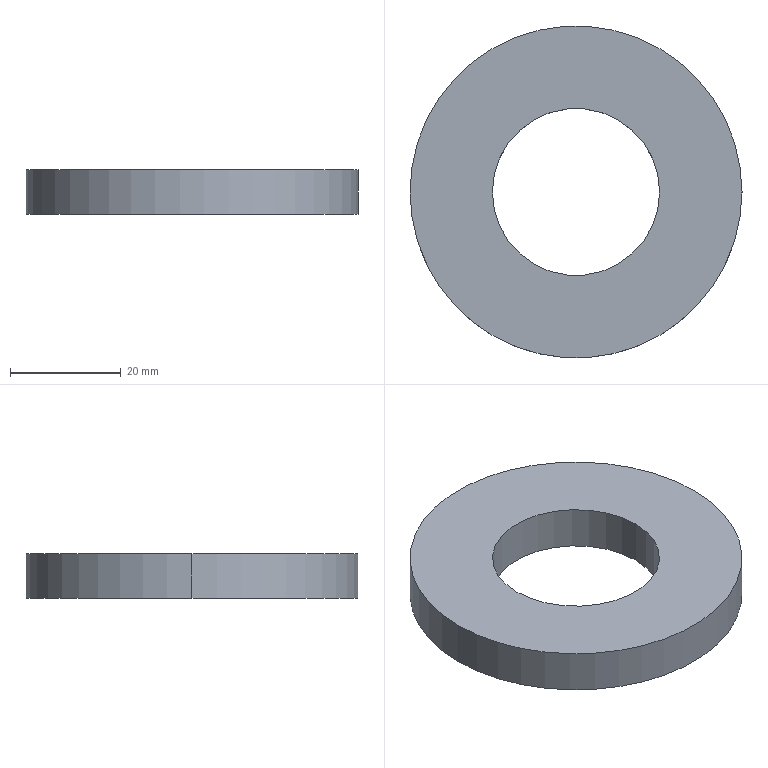Part | STEP file | LM-05-1237_default | 1 solid | 6 faces | box 60 x 60 x 8 mm | volume 16889 mm3 | cylinder 4 | plane 2 | commonest cylinder face diameters 30.2 x2 60 x2
STEP:
#1=CARTESIAN_POINT('',(0.,0.,0.));
#2=DIRECTION('',(0.,0.,1.));
#3=DIRECTION('',(1.,0.,0.));
#4=AXIS2_PLACEMENT_3D('',#1,#2,#3);
#5=CARTESIAN_POINT('',(-15.1,0.,4.));
#6=VERTEX_POINT('',#5);
#7=CARTESIAN_POINT('',(-15.1,0.,-4.));
#8=VERTEX_POINT('',#7);
#9=CARTESIAN_POINT('',(-15.1,0.,4.));
#10=DIRECTION('',(0.,0.,-1.));
#11=VECTOR('',#10,1.);
#12=LINE('',#9,#11);
#13=CARTESIAN_POINT('',(0.,0.,4.));
#14=DIRECTION('',(0.,0.,-1.));
#15=DIRECTION('',(-1.,0.,0.));
#16=AXIS2_PLACEMENT_3D('',#13,#14,#15);
#17=CYLINDRICAL_SURFACE('',#16,15.1);
#18=CARTESIAN_POINT('',(6.283,0.));
#19=DIRECTION('',(0.,1.));
#20=VECTOR('',#19,1.);
#21=LINE('',#18,#20);
#22=(GEOMETRIC_REPRESENTATION_CONTEXT(2)PARAMETRIC_REPRESENTATION_CONTEXT()REPRESENTATION_CONTEXT('',''));
#23=DEFINITIONAL_REPRESENTATION('',(#21),#22);
#24=PCURVE('',#17,#23);
#25=CARTESIAN_POINT('',(0.,0.,4.));
#26=DIRECTION('',(0.,0.,-1.));
#27=DIRECTION('',(-1.,0.,0.));
#28=AXIS2_PLACEMENT_3D('',#25,#26,#27);
#29=CYLINDRICAL_SURFACE('',#28,15.1);
#30=CARTESIAN_POINT('',(0.,0.));
#31=DIRECTION('',(0.,1.));
#32=VECTOR('',#31,1.);
#33=LINE('',#30,#32);
#34=(GEOMETRIC_REPRESENTATION_CONTEXT(2)PARAMETRIC_REPRESENTATION_CONTEXT()REPRESENTATION_CONTEXT('',''));
#35=DEFINITIONAL_REPRESENTATION('',(#33),#34);
#36=PCURVE('',#29,#35);
#37=SURFACE_CURVE('',#12,(#24,#36),.PCURVE_S1.);
#38=EDGE_CURVE('',#6,#8,#37,.T.);
#39=ORIENTED_EDGE('',*,*,#38,.T.);
#40=CARTESIAN_POINT('',(15.1,0.,-4.));
#41=VERTEX_POINT('',#40);
#42=CARTESIAN_POINT('',(0.,0.,-4.));
#43=DIRECTION('',(0.,0.,1.));
#44=DIRECTION('',(1.,0.,0.));
#45=AXIS2_PLACEMENT_3D('',#42,#43,#44);
#46=CIRCLE('',#45,15.1);
#47=CARTESIAN_POINT('',(9.425,8.));
#48=DIRECTION('',(-1.,0.));
#49=VECTOR('',#48,1.);
#50=LINE('',#47,#49);
#51=(GEOMETRIC_REPRESENTATION_CONTEXT(2)PARAMETRIC_REPRESENTATION_CONTEXT()REPRESENTATION_CONTEXT('',''));
#52=DEFINITIONAL_REPRESENTATION('',(#50),#51);
#53=PCURVE('',#17,#52);
#54=CARTESIAN_POINT('',(0.,0.,-4.));
#55=DIRECTION('',(0.,0.,1.));
#56=DIRECTION('',(1.,0.,0.));
#57=AXIS2_PLACEMENT_3D('',#54,#55,#56);
#58=PLANE('',#57);
#59=CARTESIAN_POINT('',(0.,0.));
#60=DIRECTION('',(1.,0.));
#61=AXIS2_PLACEMENT_2D('',#59,#60);
#62=CIRCLE('',#61,15.1);
#63=(GEOMETRIC_REPRESENTATION_CONTEXT(2)PARAMETRIC_REPRESENTATION_CONTEXT()REPRESENTATION_CONTEXT('',''));
#64=DEFINITIONAL_REPRESENTATION('',(#62),#63);
#65=PCURVE('',#58,#64);
#66=SURFACE_CURVE('',#46,(#53,#65),.PCURVE_S1.);
#67=EDGE_CURVE('',#8,#41,#66,.T.);
#68=ORIENTED_EDGE('',*,*,#67,.T.);
#69=CARTESIAN_POINT('',(15.1,0.,4.));
#70=VERTEX_POINT('',#69);
#71=CARTESIAN_POINT('',(15.1,0.,4.));
#72=DIRECTION('',(0.,0.,-1.));
#73=VECTOR('',#72,1.);
#74=LINE('',#71,#73);
#75=CARTESIAN_POINT('',(3.142,0.));
#76=DIRECTION('',(0.,1.));
#77=VECTOR('',#76,1.);
#78=LINE('',#75,#77);
#79=(GEOMETRIC_REPRESENTATION_CONTEXT(2)PARAMETRIC_REPRESENTATION_CONTEXT()REPRESENTATION_CONTEXT('',''));
#80=DEFINITIONAL_REPRESENTATION('',(#78),#79);
#81=PCURVE('',#17,#80);
#82=CARTESIAN_POINT('',(3.142,0.));
#83=DIRECTION('',(0.,1.));
#84=VECTOR('',#83,1.);
#85=LINE('',#82,#84);
#86=(GEOMETRIC_REPRESENTATION_CONTEXT(2)PARAMETRIC_REPRESENTATION_CONTEXT()REPRESENTATION_CONTEXT('',''));
#87=DEFINITIONAL_REPRESENTATION('',(#85),#86);
#88=PCURVE('',#29,#87);
#89=SURFACE_CURVE('',#74,(#81,#88),.PCURVE_S1.);
#90=EDGE_CURVE('',#70,#41,#89,.T.);
#91=ORIENTED_EDGE('',*,*,#90,.F.);
#92=CARTESIAN_POINT('',(0.,0.,4.));
#93=DIRECTION('',(0.,0.,1.));
#94=DIRECTION('',(1.,0.,0.));
#95=AXIS2_PLACEMENT_3D('',#92,#93,#94);
#96=CIRCLE('',#95,15.1);
#97=CARTESIAN_POINT('',(9.425,0.));
#98=DIRECTION('',(-1.,0.));
#99=VECTOR('',#98,1.);
#100=LINE('',#97,#99);
#101=(GEOMETRIC_REPRESENTATION_CONTEXT(2)PARAMETRIC_REPRESENTATION_CONTEXT()REPRESENTATION_CONTEXT('',''));
#102=DEFINITIONAL_REPRESENTATION('',(#100),#101);
#103=PCURVE('',#17,#102);
#104=CARTESIAN_POINT('',(0.,0.,4.));
#105=DIRECTION('',(0.,0.,1.));
#106=DIRECTION('',(1.,0.,0.));
#107=AXIS2_PLACEMENT_3D('',#104,#105,#106);
#108=PLANE('',#107);
#109=CARTESIAN_POINT('',(0.,0.));
#110=DIRECTION('',(1.,0.));
#111=AXIS2_PLACEMENT_2D('',#109,#110);
#112=CIRCLE('',#111,15.1);
#113=(GEOMETRIC_REPRESENTATION_CONTEXT(2)PARAMETRIC_REPRESENTATION_CONTEXT()REPRESENTATION_CONTEXT('',''));
#114=DEFINITIONAL_REPRESENTATION('',(#112),#113);
#115=PCURVE('',#108,#114);
#116=SURFACE_CURVE('',#96,(#103,#115),.PCURVE_S1.);
#117=EDGE_CURVE('',#6,#70,#116,.T.);
#118=ORIENTED_EDGE('',*,*,#117,.F.);
#119=EDGE_LOOP('',(#39,#68,#91,#118));
#120=FACE_BOUND('',#119,.F.);
#121=ADVANCED_FACE('',(#120),#17,.F.);
#122=CARTESIAN_POINT('',(30.,0.,4.));
#123=VERTEX_POINT('',#122);
#124=CARTESIAN_POINT('',(-30.,0.,4.));
#125=VERTEX_POINT('',#124);
#126=CARTESIAN_POINT('',(0.,0.,4.));
#127=DIRECTION('',(0.,0.,1.));
#128=DIRECTION('',(1.,0.,0.));
#129=AXIS2_PLACEMENT_3D('',#126,#127,#128);
#130=CIRCLE('',#129,30.);
#131=CARTESIAN_POINT('',(0.,0.,4.));
#132=DIRECTION('',(0.,0.,-1.));
#133=DIRECTION('',(-1.,0.,0.));
#134=AXIS2_PLACEMENT_3D('',#131,#132,#133);
#135=CYLINDRICAL_SURFACE('',#134,30.);
#136=CARTESIAN_POINT('',(3.142,0.));
#137=DIRECTION('',(-1.,0.));
#138=VECTOR('',#137,1.);
#139=LINE('',#136,#138);
#140=(GEOMETRIC_REPRESENTATION_CONTEXT(2)PARAMETRIC_REPRESENTATION_CONTEXT()REPRESENTATION_CONTEXT('',''));
#141=DEFINITIONAL_REPRESENTATION('',(#139),#140);
#142=PCURVE('',#135,#141);
#143=CARTESIAN_POINT('',(0.,0.));
#144=DIRECTION('',(1.,0.));
#145=AXIS2_PLACEMENT_2D('',#143,#144);
#146=CIRCLE('',#145,30.);
#147=(GEOMETRIC_REPRESENTATION_CONTEXT(2)PARAMETRIC_REPRESENTATION_CONTEXT()REPRESENTATION_CONTEXT('',''));
#148=DEFINITIONAL_REPRESENTATION('',(#146),#147);
#149=PCURVE('',#108,#148);
#150=SURFACE_CURVE('',#130,(#142,#149),.PCURVE_S1.);
#151=EDGE_CURVE('',#123,#125,#150,.T.);
#152=ORIENTED_EDGE('',*,*,#151,.F.);
#153=CARTESIAN_POINT('',(30.,0.,-4.));
#154=VERTEX_POINT('',#153);
#155=CARTESIAN_POINT('',(30.,0.,4.));
#156=DIRECTION('',(0.,0.,-1.));
#157=VECTOR('',#156,1.);
#158=LINE('',#155,#157);
#159=CARTESIAN_POINT('',(3.142,0.));
#160=DIRECTION('',(0.,1.));
#161=VECTOR('',#160,1.);
#162=LINE('',#159,#161);
#163=(GEOMETRIC_REPRESENTATION_CONTEXT(2)PARAMETRIC_REPRESENTATION_CONTEXT()REPRESENTATION_CONTEXT('',''));
#164=DEFINITIONAL_REPRESENTATION('',(#162),#163);
#165=PCURVE('',#135,#164);
#166=CARTESIAN_POINT('',(0.,0.,4.));
#167=DIRECTION('',(0.,0.,-1.));
#168=DIRECTION('',(-1.,0.,0.));
#169=AXIS2_PLACEMENT_3D('',#166,#167,#168);
#170=CYLINDRICAL_SURFACE('',#169,30.);
#171=CARTESIAN_POINT('',(3.142,0.));
#172=DIRECTION('',(0.,1.));
#173=VECTOR('',#172,1.);
#174=LINE('',#171,#173);
#175=(GEOMETRIC_REPRESENTATION_CONTEXT(2)PARAMETRIC_REPRESENTATION_CONTEXT()REPRESENTATION_CONTEXT('',''));
#176=DEFINITIONAL_REPRESENTATION('',(#174),#175);
#177=PCURVE('',#170,#176);
#178=SURFACE_CURVE('',#158,(#165,#177),.PCURVE_S1.);
#179=EDGE_CURVE('',#123,#154,#178,.T.);
#180=ORIENTED_EDGE('',*,*,#179,.T.);
#181=CARTESIAN_POINT('',(-30.,0.,-4.));
#182=VERTEX_POINT('',#181);
#183=CARTESIAN_POINT('',(0.,0.,-4.));
#184=DIRECTION('',(0.,0.,1.));
#185=DIRECTION('',(1.,0.,0.));
#186=AXIS2_PLACEMENT_3D('',#183,#184,#185);
#187=CIRCLE('',#186,30.);
#188=CARTESIAN_POINT('',(3.142,8.));
#189=DIRECTION('',(-1.,0.));
#190=VECTOR('',#189,1.);
#191=LINE('',#188,#190);
#192=(GEOMETRIC_REPRESENTATION_CONTEXT(2)PARAMETRIC_REPRESENTATION_CONTEXT()REPRESENTATION_CONTEXT('',''));
#193=DEFINITIONAL_REPRESENTATION('',(#191),#192);
#194=PCURVE('',#135,#193);
#195=CARTESIAN_POINT('',(0.,0.));
#196=DIRECTION('',(1.,0.));
#197=AXIS2_PLACEMENT_2D('',#195,#196);
#198=CIRCLE('',#197,30.);
#199=(GEOMETRIC_REPRESENTATION_CONTEXT(2)PARAMETRIC_REPRESENTATION_CONTEXT()REPRESENTATION_CONTEXT('',''));
#200=DEFINITIONAL_REPRESENTATION('',(#198),#199);
#201=PCURVE('',#58,#200);
#202=SURFACE_CURVE('',#187,(#194,#201),.PCURVE_S1.);
#203=EDGE_CURVE('',#154,#182,#202,.T.);
#204=ORIENTED_EDGE('',*,*,#203,.T.);
#205=CARTESIAN_POINT('',(-30.,0.,4.));
#206=DIRECTION('',(0.,0.,-1.));
#207=VECTOR('',#206,1.);
#208=LINE('',#205,#207);
#209=CARTESIAN_POINT('',(0.,0.));
#210=DIRECTION('',(0.,1.));
#211=VECTOR('',#210,1.);
#212=LINE('',#209,#211);
#213=(GEOMETRIC_REPRESENTATION_CONTEXT(2)PARAMETRIC_REPRESENTATION_CONTEXT()REPRESENTATION_CONTEXT('',''));
#214=DEFINITIONAL_REPRESENTATION('',(#212),#213);
#215=PCURVE('',#135,#214);
#216=CARTESIAN_POINT('',(6.283,0.));
#217=DIRECTION('',(0.,1.));
#218=VECTOR('',#217,1.);
#219=LINE('',#216,#218);
#220=(GEOMETRIC_REPRESENTATION_CONTEXT(2)PARAMETRIC_REPRESENTATION_CONTEXT()REPRESENTATION_CONTEXT('',''));
#221=DEFINITIONAL_REPRESENTATION('',(#219),#220);
#222=PCURVE('',#170,#221);
#223=SURFACE_CURVE('',#208,(#215,#222),.PCURVE_S1.);
#224=EDGE_CURVE('',#125,#182,#223,.T.);
#225=ORIENTED_EDGE('',*,*,#224,.F.);
#226=EDGE_LOOP('',(#152,#180,#204,#225));
#227=FACE_BOUND('',#226,.T.);
#228=ADVANCED_FACE('',(#227),#135,.T.);
#229=CARTESIAN_POINT('',(0.,0.,4.));
#230=DIRECTION('',(0.,0.,1.));
#231=DIRECTION('',(1.,0.,0.));
#232=AXIS2_PLACEMENT_3D('',#229,#230,#231);
#233=CIRCLE('',#232,30.);
#234=CARTESIAN_POINT('',(0.,0.));
#235=DIRECTION('',(1.,0.));
#236=AXIS2_PLACEMENT_2D('',#234,#235);
#237=CIRCLE('',#236,30.);
#238=(GEOMETRIC_REPRESENTATION_CONTEXT(2)PARAMETRIC_REPRESENTATION_CONTEXT()REPRESENTATION_CONTEXT('',''));
#239=DEFINITIONAL_REPRESENTATION('',(#237),#238);
#240=PCURVE('',#108,#239);
#241=CARTESIAN_POINT('',(9.425,0.));
#242=DIRECTION('',(-1.,0.));
#243=VECTOR('',#242,1.);
#244=LINE('',#241,#243);
#245=(GEOMETRIC_REPRESENTATION_CONTEXT(2)PARAMETRIC_REPRESENTATION_CONTEXT()REPRESENTATION_CONTEXT('',''));
#246=DEFINITIONAL_REPRESENTATION('',(#244),#245);
#247=PCURVE('',#170,#246);
#248=SURFACE_CURVE('',#233,(#240,#247),.PCURVE_S1.);
#249=EDGE_CURVE('',#125,#123,#248,.T.);
#250=ORIENTED_EDGE('',*,*,#249,.T.);
#251=ORIENTED_EDGE('',*,*,#151,.T.);
#252=EDGE_LOOP('',(#250,#251));
#253=FACE_BOUND('',#252,.T.);
#254=ORIENTED_EDGE('',*,*,#117,.F.);
#255=CARTESIAN_POINT('',(0.,0.,4.));
#256=DIRECTION('',(0.,0.,1.));
#257=DIRECTION('',(1.,0.,0.));
#258=AXIS2_PLACEMENT_3D('',#255,#256,#257);
#259=CIRCLE('',#258,15.1);
#260=CARTESIAN_POINT('',(0.,0.));
#261=DIRECTION('',(1.,0.));
#262=AXIS2_PLACEMENT_2D('',#260,#261);
#263=CIRCLE('',#262,15.1);
#264=(GEOMETRIC_REPRESENTATION_CONTEXT(2)PARAMETRIC_REPRESENTATION_CONTEXT()REPRESENTATION_CONTEXT('',''));
#265=DEFINITIONAL_REPRESENTATION('',(#263),#264);
#266=PCURVE('',#108,#265);
#267=CARTESIAN_POINT('',(3.142,0.));
#268=DIRECTION('',(-1.,0.));
#269=VECTOR('',#268,1.);
#270=LINE('',#267,#269);
#271=(GEOMETRIC_REPRESENTATION_CONTEXT(2)PARAMETRIC_REPRESENTATION_CONTEXT()REPRESENTATION_CONTEXT('',''));
#272=DEFINITIONAL_REPRESENTATION('',(#270),#271);
#273=PCURVE('',#29,#272);
#274=SURFACE_CURVE('',#259,(#266,#273),.PCURVE_S1.);
#275=EDGE_CURVE('',#70,#6,#274,.T.);
#276=ORIENTED_EDGE('',*,*,#275,.F.);
#277=EDGE_LOOP('',(#254,#276));
#278=FACE_BOUND('',#277,.T.);
#279=ADVANCED_FACE('',(#253,#278),#108,.T.);
#280=CARTESIAN_POINT('',(0.,0.,-4.));
#281=DIRECTION('',(0.,0.,1.));
#282=DIRECTION('',(1.,0.,0.));
#283=AXIS2_PLACEMENT_3D('',#280,#281,#282);
#284=CIRCLE('',#283,30.);
#285=CARTESIAN_POINT('',(0.,0.));
#286=DIRECTION('',(1.,0.));
#287=AXIS2_PLACEMENT_2D('',#285,#286);
#288=CIRCLE('',#287,30.);
#289=(GEOMETRIC_REPRESENTATION_CONTEXT(2)PARAMETRIC_REPRESENTATION_CONTEXT()REPRESENTATION_CONTEXT('',''));
#290=DEFINITIONAL_REPRESENTATION('',(#288),#289);
#291=PCURVE('',#58,#290);
#292=CARTESIAN_POINT('',(9.425,8.));
#293=DIRECTION('',(-1.,0.));
#294=VECTOR('',#293,1.);
#295=LINE('',#292,#294);
#296=(GEOMETRIC_REPRESENTATION_CONTEXT(2)PARAMETRIC_REPRESENTATION_CONTEXT()REPRESENTATION_CONTEXT('',''));
#297=DEFINITIONAL_REPRESENTATION('',(#295),#296);
#298=PCURVE('',#170,#297);
#299=SURFACE_CURVE('',#284,(#291,#298),.PCURVE_S1.);
#300=EDGE_CURVE('',#182,#154,#299,.T.);
#301=ORIENTED_EDGE('',*,*,#300,.F.);
#302=ORIENTED_EDGE('',*,*,#203,.F.);
#303=EDGE_LOOP('',(#301,#302));
#304=FACE_BOUND('',#303,.T.);
#305=ORIENTED_EDGE('',*,*,#67,.T.);
#306=CARTESIAN_POINT('',(0.,0.,-4.));
#307=DIRECTION('',(0.,0.,1.));
#308=DIRECTION('',(1.,0.,0.));
#309=AXIS2_PLACEMENT_3D('',#306,#307,#308);
#310=CIRCLE('',#309,15.1);
#311=CARTESIAN_POINT('',(0.,0.));
#312=DIRECTION('',(1.,0.));
#313=AXIS2_PLACEMENT_2D('',#311,#312);
#314=CIRCLE('',#313,15.1);
#315=(GEOMETRIC_REPRESENTATION_CONTEXT(2)PARAMETRIC_REPRESENTATION_CONTEXT()REPRESENTATION_CONTEXT('',''));
#316=DEFINITIONAL_REPRESENTATION('',(#314),#315);
#317=PCURVE('',#58,#316);
#318=CARTESIAN_POINT('',(3.142,8.));
#319=DIRECTION('',(-1.,0.));
#320=VECTOR('',#319,1.);
#321=LINE('',#318,#320);
#322=(GEOMETRIC_REPRESENTATION_CONTEXT(2)PARAMETRIC_REPRESENTATION_CONTEXT()REPRESENTATION_CONTEXT('',''));
#323=DEFINITIONAL_REPRESENTATION('',(#321),#322);
#324=PCURVE('',#29,#323);
#325=SURFACE_CURVE('',#310,(#317,#324),.PCURVE_S1.);
#326=EDGE_CURVE('',#41,#8,#325,.T.);
#327=ORIENTED_EDGE('',*,*,#326,.T.);
#328=EDGE_LOOP('',(#305,#327));
#329=FACE_BOUND('',#328,.T.);
#330=ADVANCED_FACE('',(#304,#329),#58,.F.);
#331=ORIENTED_EDGE('',*,*,#179,.F.);
#332=ORIENTED_EDGE('',*,*,#249,.F.);
#333=ORIENTED_EDGE('',*,*,#224,.T.);
#334=ORIENTED_EDGE('',*,*,#300,.T.);
#335=EDGE_LOOP('',(#331,#332,#333,#334));
#336=FACE_BOUND('',#335,.T.);
#337=ADVANCED_FACE('',(#336),#170,.T.);
#338=ORIENTED_EDGE('',*,*,#326,.T.);
#339=ORIENTED_EDGE('',*,*,#38,.F.);
#340=ORIENTED_EDGE('',*,*,#275,.F.);
#341=ORIENTED_EDGE('',*,*,#90,.T.);
#342=EDGE_LOOP('',(#338,#339,#340,#341));
#343=FACE_BOUND('',#342,.F.);
#344=ADVANCED_FACE('',(#343),#29,.F.);
#345=CLOSED_SHELL('',(#121,#228,#279,#330,#337,#344));
#346=MANIFOLD_SOLID_BREP('',#345);
#347=(LENGTH_UNIT()NAMED_UNIT(*)SI_UNIT(.MILLI.,.METRE.));
#348=UNCERTAINTY_MEASURE_WITH_UNIT(LENGTH_MEASURE(0.0000001),#347,'','');
#349=(NAMED_UNIT(*)PLANE_ANGLE_UNIT()SI_UNIT($,.RADIAN.));
#350=(NAMED_UNIT(*)SI_UNIT($,.STERADIAN.)SOLID_ANGLE_UNIT());
#351=(GEOMETRIC_REPRESENTATION_CONTEXT(3)GLOBAL_UNCERTAINTY_ASSIGNED_CONTEXT((#348))GLOBAL_UNIT_ASSIGNED_CONTEXT((#347,#349,#350))REPRESENTATION_CONTEXT('',''));
#352=ADVANCED_BREP_SHAPE_REPRESENTATION('',(#4,#346),#351);